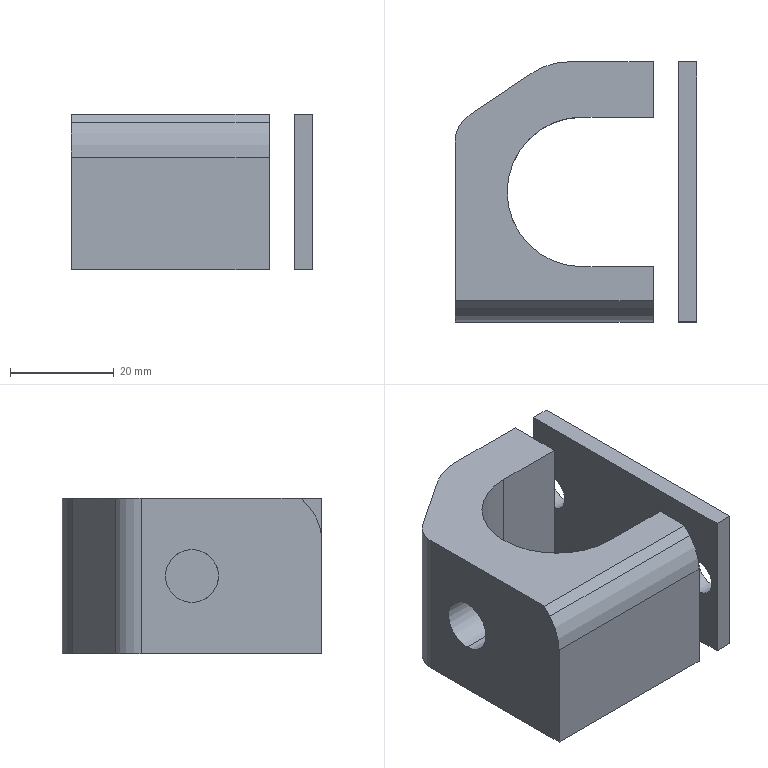Part | STEP file | SOPORTE BALANCIN | 2 solids | 36 faces | box 46.5 x 50 x 30 mm | volume 35322 mm3 | plane 17 | cylinder 15 | cone 4 | commonest cylinder face diameters 5 x4 7 x4 10.2 x2 28.8 x2 12 x1 20 x1
STEP:
#1=CARTESIAN_POINT('',(22.1,-23.5,0.));
#2=VERTEX_POINT('',#1);
#3=CARTESIAN_POINT('',(22.1,-16.5,0.));
#4=VERTEX_POINT('',#3);
#5=CARTESIAN_POINT('',(22.1,-20.,0.));
#6=DIRECTION('',(1.,0.,0.));
#7=DIRECTION('',(0.,1.,0.));
#8=AXIS2_PLACEMENT_3D('',#5,#6,#7);
#9=CIRCLE('',#8,3.5);
#10=EDGE_CURVE('',#2,#4,#9,.T.);
#11=ORIENTED_EDGE('',*,*,#10,.T.);
#12=CARTESIAN_POINT('',(18.6,-16.5,0.));
#13=VERTEX_POINT('',#12);
#14=CARTESIAN_POINT('',(22.1,-16.5,0.));
#15=DIRECTION('',(-1.,0.,0.));
#16=VECTOR('',#15,1000.);
#17=LINE('',#14,#16);
#18=EDGE_CURVE('',#4,#13,#17,.T.);
#19=ORIENTED_EDGE('',*,*,#18,.T.);
#20=CARTESIAN_POINT('',(18.6,-23.5,0.));
#21=VERTEX_POINT('',#20);
#22=CARTESIAN_POINT('',(18.6,-20.,0.));
#23=DIRECTION('',(1.,0.,0.));
#24=DIRECTION('',(0.,1.,0.));
#25=AXIS2_PLACEMENT_3D('',#22,#23,#24);
#26=CIRCLE('',#25,3.5);
#27=EDGE_CURVE('',#21,#13,#26,.T.);
#28=ORIENTED_EDGE('',*,*,#27,.F.);
#29=CARTESIAN_POINT('',(22.1,-23.5,0.));
#30=DIRECTION('',(-1.,0.,0.));
#31=VECTOR('',#30,1000.);
#32=LINE('',#29,#31);
#33=EDGE_CURVE('',#2,#21,#32,.T.);
#34=ORIENTED_EDGE('',*,*,#33,.F.);
#35=EDGE_LOOP('',(#11,#19,#28,#34));
#36=FACE_OUTER_BOUND('',#35,.T.);
#37=CARTESIAN_POINT('',(22.1,-20.,0.));
#38=DIRECTION('',(-1.,0.,0.));
#39=DIRECTION('',(0.,-1.,0.));
#40=AXIS2_PLACEMENT_3D('',#37,#38,#39);
#41=CYLINDRICAL_SURFACE('',#40,3.5);
#42=ADVANCED_FACE('',(#36),#41,.F.);
#43=CARTESIAN_POINT('',(22.1,16.5,0.));
#44=VERTEX_POINT('',#43);
#45=CARTESIAN_POINT('',(22.1,23.5,0.));
#46=VERTEX_POINT('',#45);
#47=CARTESIAN_POINT('',(22.1,20.,0.));
#48=DIRECTION('',(1.,0.,0.));
#49=DIRECTION('',(0.,1.,0.));
#50=AXIS2_PLACEMENT_3D('',#47,#48,#49);
#51=CIRCLE('',#50,3.5);
#52=EDGE_CURVE('',#44,#46,#51,.T.);
#53=ORIENTED_EDGE('',*,*,#52,.T.);
#54=CARTESIAN_POINT('',(18.6,23.5,0.));
#55=VERTEX_POINT('',#54);
#56=CARTESIAN_POINT('',(22.1,23.5,0.));
#57=DIRECTION('',(-1.,0.,0.));
#58=VECTOR('',#57,1000.);
#59=LINE('',#56,#58);
#60=EDGE_CURVE('',#46,#55,#59,.T.);
#61=ORIENTED_EDGE('',*,*,#60,.T.);
#62=CARTESIAN_POINT('',(18.6,16.5,0.));
#63=VERTEX_POINT('',#62);
#64=CARTESIAN_POINT('',(18.6,20.,0.));
#65=DIRECTION('',(1.,0.,0.));
#66=DIRECTION('',(0.,1.,0.));
#67=AXIS2_PLACEMENT_3D('',#64,#65,#66);
#68=CIRCLE('',#67,3.5);
#69=EDGE_CURVE('',#63,#55,#68,.T.);
#70=ORIENTED_EDGE('',*,*,#69,.F.);
#71=CARTESIAN_POINT('',(22.1,16.5,0.));
#72=DIRECTION('',(-1.,0.,0.));
#73=VECTOR('',#72,1000.);
#74=LINE('',#71,#73);
#75=EDGE_CURVE('',#44,#63,#74,.T.);
#76=ORIENTED_EDGE('',*,*,#75,.F.);
#77=EDGE_LOOP('',(#53,#61,#70,#76));
#78=FACE_OUTER_BOUND('',#77,.T.);
#79=CARTESIAN_POINT('',(22.1,20.,0.));
#80=DIRECTION('',(-1.,0.,0.));
#81=DIRECTION('',(0.,-1.,0.));
#82=AXIS2_PLACEMENT_3D('',#79,#80,#81);
#83=CYLINDRICAL_SURFACE('',#82,3.5);
#84=ADVANCED_FACE('',(#78),#83,.F.);
#85=CARTESIAN_POINT('',(22.1,-25.,-15.));
#86=VERTEX_POINT('',#85);
#87=CARTESIAN_POINT('',(22.1,25.,-15.));
#88=VERTEX_POINT('',#87);
#89=CARTESIAN_POINT('',(22.1,-25.,-15.));
#90=DIRECTION('',(0.,1.,0.));
#91=VECTOR('',#90,1000.);
#92=LINE('',#89,#91);
#93=EDGE_CURVE('',#86,#88,#92,.T.);
#94=ORIENTED_EDGE('',*,*,#93,.T.);
#95=CARTESIAN_POINT('',(22.1,25.,15.));
#96=VERTEX_POINT('',#95);
#97=CARTESIAN_POINT('',(22.1,25.,15.));
#98=DIRECTION('',(0.,0.,1.));
#99=VECTOR('',#98,1000.);
#100=LINE('',#97,#99);
#101=EDGE_CURVE('',#88,#96,#100,.T.);
#102=ORIENTED_EDGE('',*,*,#101,.T.);
#103=CARTESIAN_POINT('',(22.1,-25.,15.));
#104=VERTEX_POINT('',#103);
#105=CARTESIAN_POINT('',(22.1,-25.,15.));
#106=DIRECTION('',(0.,-1.,0.));
#107=VECTOR('',#106,1000.);
#108=LINE('',#105,#107);
#109=EDGE_CURVE('',#96,#104,#108,.T.);
#110=ORIENTED_EDGE('',*,*,#109,.T.);
#111=CARTESIAN_POINT('',(22.1,-25.,15.));
#112=DIRECTION('',(0.,0.,-1.));
#113=VECTOR('',#112,1000.);
#114=LINE('',#111,#113);
#115=EDGE_CURVE('',#104,#86,#114,.T.);
#116=ORIENTED_EDGE('',*,*,#115,.T.);
#117=EDGE_LOOP('',(#94,#102,#110,#116));
#118=FACE_OUTER_BOUND('',#117,.T.);
#119=ORIENTED_EDGE('',*,*,#52,.F.);
#120=CARTESIAN_POINT('',(22.1,20.,0.));
#121=DIRECTION('',(1.,0.,0.));
#122=DIRECTION('',(0.,1.,0.));
#123=AXIS2_PLACEMENT_3D('',#120,#121,#122);
#124=CIRCLE('',#123,3.5);
#125=EDGE_CURVE('',#46,#44,#124,.T.);
#126=ORIENTED_EDGE('',*,*,#125,.F.);
#127=EDGE_LOOP('',(#119,#126));
#128=FACE_BOUND('',#127,.T.);
#129=ORIENTED_EDGE('',*,*,#10,.F.);
#130=CARTESIAN_POINT('',(22.1,-20.,0.));
#131=DIRECTION('',(1.,0.,0.));
#132=DIRECTION('',(0.,1.,0.));
#133=AXIS2_PLACEMENT_3D('',#130,#131,#132);
#134=CIRCLE('',#133,3.5);
#135=EDGE_CURVE('',#4,#2,#134,.T.);
#136=ORIENTED_EDGE('',*,*,#135,.F.);
#137=EDGE_LOOP('',(#129,#136));
#138=FACE_BOUND('',#137,.T.);
#139=CARTESIAN_POINT('',(22.1,0.,0.));
#140=DIRECTION('',(-1.,0.,0.));
#141=DIRECTION('',(0.,-1.,0.));
#142=AXIS2_PLACEMENT_3D('',#139,#140,#141);
#143=PLANE('',#142);
#144=ADVANCED_FACE('',(#118,#128,#138),#143,.F.);
#145=ORIENTED_EDGE('',*,*,#69,.T.);
#146=CARTESIAN_POINT('',(18.6,20.,0.));
#147=DIRECTION('',(1.,0.,0.));
#148=DIRECTION('',(0.,1.,0.));
#149=AXIS2_PLACEMENT_3D('',#146,#147,#148);
#150=CIRCLE('',#149,3.5);
#151=EDGE_CURVE('',#55,#63,#150,.T.);
#152=ORIENTED_EDGE('',*,*,#151,.T.);
#153=EDGE_LOOP('',(#145,#152));
#154=FACE_BOUND('',#153,.T.);
#155=CARTESIAN_POINT('',(18.6,-25.,-15.));
#156=VERTEX_POINT('',#155);
#157=CARTESIAN_POINT('',(18.6,25.,-15.));
#158=VERTEX_POINT('',#157);
#159=CARTESIAN_POINT('',(18.6,-25.,-15.));
#160=DIRECTION('',(0.,1.,0.));
#161=VECTOR('',#160,1000.);
#162=LINE('',#159,#161);
#163=EDGE_CURVE('',#156,#158,#162,.T.);
#164=ORIENTED_EDGE('',*,*,#163,.F.);
#165=CARTESIAN_POINT('',(18.6,-25.,15.));
#166=VERTEX_POINT('',#165);
#167=CARTESIAN_POINT('',(18.6,-25.,15.));
#168=DIRECTION('',(0.,0.,-1.));
#169=VECTOR('',#168,1000.);
#170=LINE('',#167,#169);
#171=EDGE_CURVE('',#166,#156,#170,.T.);
#172=ORIENTED_EDGE('',*,*,#171,.F.);
#173=CARTESIAN_POINT('',(18.6,25.,15.));
#174=VERTEX_POINT('',#173);
#175=CARTESIAN_POINT('',(18.6,-25.,15.));
#176=DIRECTION('',(0.,-1.,0.));
#177=VECTOR('',#176,1000.);
#178=LINE('',#175,#177);
#179=EDGE_CURVE('',#174,#166,#178,.T.);
#180=ORIENTED_EDGE('',*,*,#179,.F.);
#181=CARTESIAN_POINT('',(18.6,25.,15.));
#182=DIRECTION('',(0.,0.,1.));
#183=VECTOR('',#182,1000.);
#184=LINE('',#181,#183);
#185=EDGE_CURVE('',#158,#174,#184,.T.);
#186=ORIENTED_EDGE('',*,*,#185,.F.);
#187=EDGE_LOOP('',(#164,#172,#180,#186));
#188=FACE_OUTER_BOUND('',#187,.T.);
#189=ORIENTED_EDGE('',*,*,#27,.T.);
#190=CARTESIAN_POINT('',(18.6,-20.,0.));
#191=DIRECTION('',(1.,0.,0.));
#192=DIRECTION('',(0.,1.,0.));
#193=AXIS2_PLACEMENT_3D('',#190,#191,#192);
#194=CIRCLE('',#193,3.5);
#195=EDGE_CURVE('',#13,#21,#194,.T.);
#196=ORIENTED_EDGE('',*,*,#195,.T.);
#197=EDGE_LOOP('',(#189,#196));
#198=FACE_BOUND('',#197,.T.);
#199=CARTESIAN_POINT('',(18.6,0.,0.));
#200=DIRECTION('',(-1.,0.,0.));
#201=DIRECTION('',(0.,-1.,0.));
#202=AXIS2_PLACEMENT_3D('',#199,#200,#201);
#203=PLANE('',#202);
#204=ADVANCED_FACE('',(#154,#188,#198),#203,.T.);
#205=ORIENTED_EDGE('',*,*,#163,.T.);
#206=CARTESIAN_POINT('',(22.1,25.,-15.));
#207=DIRECTION('',(-1.,0.,0.));
#208=VECTOR('',#207,1000.);
#209=LINE('',#206,#208);
#210=EDGE_CURVE('',#88,#158,#209,.T.);
#211=ORIENTED_EDGE('',*,*,#210,.F.);
#212=ORIENTED_EDGE('',*,*,#93,.F.);
#213=CARTESIAN_POINT('',(22.1,-25.,-15.));
#214=DIRECTION('',(-1.,0.,0.));
#215=VECTOR('',#214,1000.);
#216=LINE('',#213,#215);
#217=EDGE_CURVE('',#86,#156,#216,.T.);
#218=ORIENTED_EDGE('',*,*,#217,.T.);
#219=EDGE_LOOP('',(#205,#211,#212,#218));
#220=FACE_OUTER_BOUND('',#219,.T.);
#221=CARTESIAN_POINT('',(22.1,-25.,-15.));
#222=DIRECTION('',(0.,0.,1.));
#223=DIRECTION('',(1.,0.,0.));
#224=AXIS2_PLACEMENT_3D('',#221,#222,#223);
#225=PLANE('',#224);
#226=ADVANCED_FACE('',(#220),#225,.F.);
#227=ORIENTED_EDGE('',*,*,#185,.T.);
#228=CARTESIAN_POINT('',(22.1,25.,15.));
#229=DIRECTION('',(-1.,0.,0.));
#230=VECTOR('',#229,1000.);
#231=LINE('',#228,#230);
#232=EDGE_CURVE('',#96,#174,#231,.T.);
#233=ORIENTED_EDGE('',*,*,#232,.F.);
#234=ORIENTED_EDGE('',*,*,#101,.F.);
#235=ORIENTED_EDGE('',*,*,#210,.T.);
#236=EDGE_LOOP('',(#227,#233,#234,#235));
#237=FACE_OUTER_BOUND('',#236,.T.);
#238=CARTESIAN_POINT('',(22.1,25.,15.));
#239=DIRECTION('',(0.,-1.,0.));
#240=DIRECTION('',(1.,0.,0.));
#241=AXIS2_PLACEMENT_3D('',#238,#239,#240);
#242=PLANE('',#241);
#243=ADVANCED_FACE('',(#237),#242,.F.);
#244=ORIENTED_EDGE('',*,*,#179,.T.);
#245=CARTESIAN_POINT('',(22.1,-25.,15.));
#246=DIRECTION('',(-1.,0.,0.));
#247=VECTOR('',#246,1000.);
#248=LINE('',#245,#247);
#249=EDGE_CURVE('',#104,#166,#248,.T.);
#250=ORIENTED_EDGE('',*,*,#249,.F.);
#251=ORIENTED_EDGE('',*,*,#109,.F.);
#252=ORIENTED_EDGE('',*,*,#232,.T.);
#253=EDGE_LOOP('',(#244,#250,#251,#252));
#254=FACE_OUTER_BOUND('',#253,.T.);
#255=CARTESIAN_POINT('',(22.1,-25.,15.));
#256=DIRECTION('',(0.,0.,-1.));
#257=DIRECTION('',(-1.,0.,0.));
#258=AXIS2_PLACEMENT_3D('',#255,#256,#257);
#259=PLANE('',#258);
#260=ADVANCED_FACE('',(#254),#259,.F.);
#261=ORIENTED_EDGE('',*,*,#171,.T.);
#262=ORIENTED_EDGE('',*,*,#217,.F.);
#263=ORIENTED_EDGE('',*,*,#115,.F.);
#264=ORIENTED_EDGE('',*,*,#249,.T.);
#265=EDGE_LOOP('',(#261,#262,#263,#264));
#266=FACE_OUTER_BOUND('',#265,.T.);
#267=CARTESIAN_POINT('',(22.1,-25.,15.));
#268=DIRECTION('',(0.,1.,0.));
#269=DIRECTION('',(-1.,0.,0.));
#270=AXIS2_PLACEMENT_3D('',#267,#268,#269);
#271=PLANE('',#270);
#272=ADVANCED_FACE('',(#266),#271,.F.);
#273=ORIENTED_EDGE('',*,*,#60,.F.);
#274=ORIENTED_EDGE('',*,*,#125,.T.);
#275=ORIENTED_EDGE('',*,*,#75,.T.);
#276=ORIENTED_EDGE('',*,*,#151,.F.);
#277=EDGE_LOOP('',(#273,#274,#275,#276));
#278=FACE_OUTER_BOUND('',#277,.T.);
#279=CARTESIAN_POINT('',(22.1,20.,0.));
#280=DIRECTION('',(-1.,0.,0.));
#281=DIRECTION('',(0.,-1.,0.));
#282=AXIS2_PLACEMENT_3D('',#279,#280,#281);
#283=CYLINDRICAL_SURFACE('',#282,3.5);
#284=ADVANCED_FACE('',(#278),#283,.F.);
#285=ORIENTED_EDGE('',*,*,#18,.F.);
#286=ORIENTED_EDGE('',*,*,#135,.T.);
#287=ORIENTED_EDGE('',*,*,#33,.T.);
#288=ORIENTED_EDGE('',*,*,#195,.F.);
#289=EDGE_LOOP('',(#285,#286,#287,#288));
#290=FACE_OUTER_BOUND('',#289,.T.);
#291=CARTESIAN_POINT('',(22.1,-20.,0.));
#292=DIRECTION('',(-1.,0.,0.));
#293=DIRECTION('',(0.,-1.,0.));
#294=AXIS2_PLACEMENT_3D('',#291,#292,#293);
#295=CYLINDRICAL_SURFACE('',#294,3.5);
#296=ADVANCED_FACE('',(#290),#295,.F.);
#297=CLOSED_SHELL('',(#42,#84,#144,#204,#226,#243,#260,#272,#284,#296));
#298=MANIFOLD_SOLID_BREP('',#297);
#299=CARTESIAN_POINT('',(-14.4,0.,-5.1));
#300=VERTEX_POINT('',#299);
#301=CARTESIAN_POINT('',(-14.4,0.,5.1));
#302=VERTEX_POINT('',#301);
#303=CARTESIAN_POINT('',(-14.4,0.,-5.1));
#304=CARTESIAN_POINT('',(-14.4,-0.1674,-5.1));
#305=CARTESIAN_POINT('',(-14.397,-0.3348,-5.092));
#306=CARTESIAN_POINT('',(-14.385,-0.6696,-5.059));
#307=CARTESIAN_POINT('',(-14.377,-0.838,-5.034));
#308=CARTESIAN_POINT('',(-14.342,-1.334,-4.934));
#309=CARTESIAN_POINT('',(-14.308,-1.653,-4.836));
#310=CARTESIAN_POINT('',(-14.224,-2.269,-4.58));
#311=CARTESIAN_POINT('',(-14.172,-2.567,-4.419));
#312=CARTESIAN_POINT('',(-14.061,-3.117,-4.05));
#313=CARTESIAN_POINT('',(-14.002,-3.372,-3.84));
#314=CARTESIAN_POINT('',(-13.88,-3.843,-3.369));
#315=CARTESIAN_POINT('',(-13.819,-4.054,-3.112));
#316=CARTESIAN_POINT('',(-13.734,-4.329,-2.701));
#317=CARTESIAN_POINT('',(-13.707,-4.415,-2.559));
#318=CARTESIAN_POINT('',(-13.655,-4.572,-2.266));
#319=CARTESIAN_POINT('',(-13.631,-4.645,-2.113));
#320=CARTESIAN_POINT('',(-13.564,-4.838,-1.649));
#321=CARTESIAN_POINT('',(-13.528,-4.935,-1.331));
#322=CARTESIAN_POINT('',(-13.48,-5.066,-0.6757));
#323=CARTESIAN_POINT('',(-13.467,-5.1,-0.3347));
#324=CARTESIAN_POINT('',(-13.467,-5.1,0.3374));
#325=CARTESIAN_POINT('',(-13.479,-5.067,0.6706));
#326=CARTESIAN_POINT('',(-13.516,-4.968,1.166));
#327=CARTESIAN_POINT('',(-13.531,-4.926,1.331));
#328=CARTESIAN_POINT('',(-13.567,-4.828,1.651));
#329=CARTESIAN_POINT('',(-13.587,-4.772,1.808));
#330=CARTESIAN_POINT('',(-13.653,-4.58,2.269));
#331=CARTESIAN_POINT('',(-13.706,-4.421,2.565));
#332=CARTESIAN_POINT('',(-13.82,-4.05,3.118));
#333=CARTESIAN_POINT('',(-13.881,-3.84,3.373));
#334=CARTESIAN_POINT('',(-14.002,-3.372,3.84));
#335=CARTESIAN_POINT('',(-14.062,-3.112,4.054));
#336=CARTESIAN_POINT('',(-14.173,-2.562,4.422));
#337=CARTESIAN_POINT('',(-14.223,-2.27,4.579));
#338=CARTESIAN_POINT('',(-14.287,-1.807,4.772));
#339=CARTESIAN_POINT('',(-14.306,-1.647,4.83));
#340=CARTESIAN_POINT('',(-14.34,-1.326,4.927));
#341=CARTESIAN_POINT('',(-14.354,-1.164,4.968));
#342=CARTESIAN_POINT('',(-14.388,-0.6735,5.066));
#343=CARTESIAN_POINT('',(-14.4,-0.3399,5.1));
#344=CARTESIAN_POINT('',(-14.4,0.,5.1));
#345=B_SPLINE_CURVE_WITH_KNOTS('',3,(#303,#304,#305,#306,#307,#308,#309,#310,#311,#312,#313,#314,#315,#316,#317,#318,#319,#320,#321,#322,#323,#324,#325,#326,#327,#328,#329,#330,#331,#332,#333,#334,#335,#336,#337,#338,#339,#340,#341,#342,#343,#344),.UNSPECIFIED.,.F.,.F.,(4,2,2,2,2,2,2,2,2,2,2,2,2,2,2,2,2,2,2,2,4),(0.01608,0.01658,0.01708,0.01809,0.01909,0.02009,0.0211,0.0216,0.0221,0.02311,0.02411,0.02512,0.02562,0.02612,0.02713,0.02813,0.02914,0.03014,0.03064,0.03114,0.03215),.UNSPECIFIED.);
#346=EDGE_CURVE('',#300,#302,#345,.T.);
#347=ORIENTED_EDGE('',*,*,#346,.F.);
#348=CARTESIAN_POINT('',(-24.4,0.,-5.1));
#349=VERTEX_POINT('',#348);
#350=CARTESIAN_POINT('',(-24.4,0.,-5.1));
#351=DIRECTION('',(-1.,0.,0.));
#352=VECTOR('',#351,1000.);
#353=LINE('',#350,#352);
#354=EDGE_CURVE('',#300,#349,#353,.T.);
#355=ORIENTED_EDGE('',*,*,#354,.T.);
#356=CARTESIAN_POINT('',(-24.4,0.,5.1));
#357=VERTEX_POINT('',#356);
#358=CARTESIAN_POINT('',(-24.4,0.,0.));
#359=DIRECTION('',(-1.,0.,0.));
#360=DIRECTION('',(0.,0.,1.));
#361=AXIS2_PLACEMENT_3D('',#358,#359,#360);
#362=CIRCLE('',#361,5.1);
#363=EDGE_CURVE('',#349,#357,#362,.T.);
#364=ORIENTED_EDGE('',*,*,#363,.T.);
#365=CARTESIAN_POINT('',(-24.4,0.,5.1));
#366=DIRECTION('',(-1.,0.,0.));
#367=VECTOR('',#366,1000.);
#368=LINE('',#365,#367);
#369=EDGE_CURVE('',#302,#357,#368,.T.);
#370=ORIENTED_EDGE('',*,*,#369,.F.);
#371=EDGE_LOOP('',(#347,#355,#364,#370));
#372=FACE_OUTER_BOUND('',#371,.T.);
#373=CARTESIAN_POINT('',(-24.4,0.,0.));
#374=DIRECTION('',(-1.,0.,0.));
#375=DIRECTION('',(0.,0.,1.));
#376=AXIS2_PLACEMENT_3D('',#373,#374,#375);
#377=CYLINDRICAL_SURFACE('',#376,5.1);
#378=ADVANCED_FACE('',(#372),#377,.F.);
#379=CARTESIAN_POINT('',(-1.898,20.,2.5));
#380=VERTEX_POINT('',#379);
#381=CARTESIAN_POINT('',(-1.898,20.,-2.5));
#382=VERTEX_POINT('',#381);
#383=CARTESIAN_POINT('',(-1.898,20.,0.));
#384=DIRECTION('',(1.,0.,0.));
#385=DIRECTION('',(0.,0.,-1.));
#386=AXIS2_PLACEMENT_3D('',#383,#384,#385);
#387=CIRCLE('',#386,2.5);
#388=EDGE_CURVE('',#380,#382,#387,.T.);
#389=ORIENTED_EDGE('',*,*,#388,.F.);
#390=CARTESIAN_POINT('',(13.7,20.,2.5));
#391=VERTEX_POINT('',#390);
#392=CARTESIAN_POINT('',(13.6,20.,2.5));
#393=DIRECTION('',(1.,0.,0.));
#394=VECTOR('',#393,1000.);
#395=LINE('',#392,#394);
#396=EDGE_CURVE('',#380,#391,#395,.T.);
#397=ORIENTED_EDGE('',*,*,#396,.T.);
#398=CARTESIAN_POINT('',(13.7,20.,-2.5));
#399=VERTEX_POINT('',#398);
#400=CARTESIAN_POINT('',(13.7,20.,0.));
#401=DIRECTION('',(1.,0.,0.));
#402=DIRECTION('',(0.,-1.,0.));
#403=AXIS2_PLACEMENT_3D('',#400,#401,#402);
#404=CIRCLE('',#403,2.5);
#405=EDGE_CURVE('',#391,#399,#404,.T.);
#406=ORIENTED_EDGE('',*,*,#405,.T.);
#407=CARTESIAN_POINT('',(13.6,20.,-2.5));
#408=DIRECTION('',(1.,0.,0.));
#409=VECTOR('',#408,1000.);
#410=LINE('',#407,#409);
#411=EDGE_CURVE('',#382,#399,#410,.T.);
#412=ORIENTED_EDGE('',*,*,#411,.F.);
#413=EDGE_LOOP('',(#389,#397,#406,#412));
#414=FACE_OUTER_BOUND('',#413,.T.);
#415=CARTESIAN_POINT('',(13.6,20.,0.));
#416=DIRECTION('',(1.,0.,0.));
#417=DIRECTION('',(0.,0.,-1.));
#418=AXIS2_PLACEMENT_3D('',#415,#416,#417);
#419=CYLINDRICAL_SURFACE('',#418,2.5);
#420=ADVANCED_FACE('',(#414),#419,.F.);
#421=CARTESIAN_POINT('',(-3.4,20.,0.));
#422=VERTEX_POINT('',#421);
#423=CARTESIAN_POINT('',(-1.898,20.,-2.5));
#424=DIRECTION('',(0.515,0.,-0.8572));
#425=VECTOR('',#424,1000.);
#426=LINE('',#423,#425);
#427=EDGE_CURVE('',#422,#382,#426,.T.);
#428=ORIENTED_EDGE('',*,*,#427,.F.);
#429=CARTESIAN_POINT('',(-1.898,20.,2.5));
#430=DIRECTION('',(0.515,0.,0.8572));
#431=VECTOR('',#430,1000.);
#432=LINE('',#429,#431);
#433=EDGE_CURVE('',#422,#380,#432,.T.);
#434=ORIENTED_EDGE('',*,*,#433,.T.);
#435=ORIENTED_EDGE('',*,*,#388,.T.);
#436=EDGE_LOOP('',(#428,#434,#435));
#437=FACE_OUTER_BOUND('',#436,.T.);
#438=CARTESIAN_POINT('',(-1.898,20.,0.));
#439=DIRECTION('',(1.,0.,0.));
#440=DIRECTION('',(0.,0.,-1.));
#441=AXIS2_PLACEMENT_3D('',#438,#439,#440);
#442=CONICAL_SURFACE('',#441,2.5,1.03);
#443=ADVANCED_FACE('',(#437),#442,.F.);
#444=CARTESIAN_POINT('',(-1.898,-20.,2.5));
#445=VERTEX_POINT('',#444);
#446=CARTESIAN_POINT('',(-1.898,-20.,-2.5));
#447=VERTEX_POINT('',#446);
#448=CARTESIAN_POINT('',(-1.898,-20.,0.));
#449=DIRECTION('',(1.,0.,0.));
#450=DIRECTION('',(0.,0.,-1.));
#451=AXIS2_PLACEMENT_3D('',#448,#449,#450);
#452=CIRCLE('',#451,2.5);
#453=EDGE_CURVE('',#445,#447,#452,.T.);
#454=ORIENTED_EDGE('',*,*,#453,.F.);
#455=CARTESIAN_POINT('',(13.7,-20.,2.5));
#456=VERTEX_POINT('',#455);
#457=CARTESIAN_POINT('',(13.6,-20.,2.5));
#458=DIRECTION('',(1.,0.,0.));
#459=VECTOR('',#458,1000.);
#460=LINE('',#457,#459);
#461=EDGE_CURVE('',#445,#456,#460,.T.);
#462=ORIENTED_EDGE('',*,*,#461,.T.);
#463=CARTESIAN_POINT('',(13.7,-20.,-2.5));
#464=VERTEX_POINT('',#463);
#465=CARTESIAN_POINT('',(13.7,-20.,0.));
#466=DIRECTION('',(1.,0.,0.));
#467=DIRECTION('',(0.,-1.,0.));
#468=AXIS2_PLACEMENT_3D('',#465,#466,#467);
#469=CIRCLE('',#468,2.5);
#470=EDGE_CURVE('',#456,#464,#469,.T.);
#471=ORIENTED_EDGE('',*,*,#470,.T.);
#472=CARTESIAN_POINT('',(13.6,-20.,-2.5));
#473=DIRECTION('',(1.,0.,0.));
#474=VECTOR('',#473,1000.);
#475=LINE('',#472,#474);
#476=EDGE_CURVE('',#447,#464,#475,.T.);
#477=ORIENTED_EDGE('',*,*,#476,.F.);
#478=EDGE_LOOP('',(#454,#462,#471,#477));
#479=FACE_OUTER_BOUND('',#478,.T.);
#480=CARTESIAN_POINT('',(13.6,-20.,0.));
#481=DIRECTION('',(1.,0.,0.));
#482=DIRECTION('',(0.,0.,-1.));
#483=AXIS2_PLACEMENT_3D('',#480,#481,#482);
#484=CYLINDRICAL_SURFACE('',#483,2.5);
#485=ADVANCED_FACE('',(#479),#484,.F.);
#486=CARTESIAN_POINT('',(-3.4,-20.,0.));
#487=VERTEX_POINT('',#486);
#488=CARTESIAN_POINT('',(-1.898,-20.,-2.5));
#489=DIRECTION('',(0.515,0.,-0.8572));
#490=VECTOR('',#489,1000.);
#491=LINE('',#488,#490);
#492=EDGE_CURVE('',#487,#447,#491,.T.);
#493=ORIENTED_EDGE('',*,*,#492,.F.);
#494=CARTESIAN_POINT('',(-1.898,-20.,2.5));
#495=DIRECTION('',(0.515,0.,0.8572));
#496=VECTOR('',#495,1000.);
#497=LINE('',#494,#496);
#498=EDGE_CURVE('',#487,#445,#497,.T.);
#499=ORIENTED_EDGE('',*,*,#498,.T.);
#500=ORIENTED_EDGE('',*,*,#453,.T.);
#501=EDGE_LOOP('',(#493,#499,#500));
#502=FACE_OUTER_BOUND('',#501,.T.);
#503=CARTESIAN_POINT('',(-1.898,-20.,0.));
#504=DIRECTION('',(1.,0.,0.));
#505=DIRECTION('',(0.,0.,-1.));
#506=AXIS2_PLACEMENT_3D('',#503,#504,#505);
#507=CONICAL_SURFACE('',#506,2.5,1.03);
#508=ADVANCED_FACE('',(#502),#507,.F.);
#509=CARTESIAN_POINT('',(-14.4,0.,15.));
#510=VERTEX_POINT('',#509);
#511=CARTESIAN_POINT('',(0.,14.4,15.));
#512=VERTEX_POINT('',#511);
#513=CARTESIAN_POINT('',(0.,0.,15.));
#514=DIRECTION('',(0.,0.,-1.));
#515=DIRECTION('',(1.,0.,0.));
#516=AXIS2_PLACEMENT_3D('',#513,#514,#515);
#517=CIRCLE('',#516,14.4);
#518=EDGE_CURVE('',#510,#512,#517,.T.);
#519=ORIENTED_EDGE('',*,*,#518,.F.);
#520=CARTESIAN_POINT('',(-14.4,0.,15.));
#521=DIRECTION('',(0.,0.,-1.));
#522=VECTOR('',#521,1000.);
#523=LINE('',#520,#522);
#524=EDGE_CURVE('',#510,#302,#523,.T.);
#525=ORIENTED_EDGE('',*,*,#524,.T.);
#526=CARTESIAN_POINT('',(-14.4,0.,5.1));
#527=CARTESIAN_POINT('',(-14.4,0.3399,5.1));
#528=CARTESIAN_POINT('',(-14.388,0.6737,5.066));
#529=CARTESIAN_POINT('',(-14.342,1.329,4.935));
#530=CARTESIAN_POINT('',(-14.308,1.655,4.836));
#531=CARTESIAN_POINT('',(-14.223,2.271,4.578));
#532=CARTESIAN_POINT('',(-14.173,2.563,4.421));
#533=CARTESIAN_POINT('',(-14.062,3.116,4.051));
#534=CARTESIAN_POINT('',(-14.001,3.375,3.838));
#535=CARTESIAN_POINT('',(-13.88,3.841,3.371));
#536=CARTESIAN_POINT('',(-13.82,4.051,3.116));
#537=CARTESIAN_POINT('',(-13.705,4.424,2.56));
#538=CARTESIAN_POINT('',(-13.653,4.58,2.268));
#539=CARTESIAN_POINT('',(-13.587,4.772,1.808));
#540=CARTESIAN_POINT('',(-13.567,4.828,1.652));
#541=CARTESIAN_POINT('',(-13.531,4.926,1.331));
#542=CARTESIAN_POINT('',(-13.516,4.968,1.166));
#543=CARTESIAN_POINT('',(-13.479,5.067,0.6712));
#544=CARTESIAN_POINT('',(-13.467,5.1,0.3384));
#545=CARTESIAN_POINT('',(-13.467,5.1,-0.3331));
#546=CARTESIAN_POINT('',(-13.48,5.066,-0.6741));
#547=CARTESIAN_POINT('',(-13.528,4.935,-1.331));
#548=CARTESIAN_POINT('',(-13.564,4.837,-1.65));
#549=CARTESIAN_POINT('',(-13.653,4.579,-2.271));
#550=CARTESIAN_POINT('',(-13.706,4.421,-2.564));
#551=CARTESIAN_POINT('',(-13.819,4.053,-3.114));
#552=CARTESIAN_POINT('',(-13.881,3.839,-3.373));
#553=CARTESIAN_POINT('',(-14.002,3.37,-3.842));
#554=CARTESIAN_POINT('',(-14.062,3.116,-4.051));
#555=CARTESIAN_POINT('',(-14.173,2.565,-4.421));
#556=CARTESIAN_POINT('',(-14.224,2.266,-4.581));
#557=CARTESIAN_POINT('',(-14.308,1.653,-4.836));
#558=CARTESIAN_POINT('',(-14.342,1.334,-4.934));
#559=CARTESIAN_POINT('',(-14.377,0.838,-5.034));
#560=CARTESIAN_POINT('',(-14.385,0.6696,-5.059));
#561=CARTESIAN_POINT('',(-14.397,0.3348,-5.092));
#562=CARTESIAN_POINT('',(-14.4,0.1674,-5.1));
#563=CARTESIAN_POINT('',(-14.4,0.,-5.1));
#564=B_SPLINE_CURVE_WITH_KNOTS('',3,(#526,#527,#528,#529,#530,#531,#532,#533,#534,#535,#536,#537,#538,#539,#540,#541,#542,#543,#544,#545,#546,#547,#548,#549,#550,#551,#552,#553,#554,#555,#556,#557,#558,#559,#560,#561,#562,#563),.UNSPECIFIED.,.F.,.F.,(4,2,2,2,2,2,2,2,2,2,2,2,2,2,2,2,2,2,4),(0.,0.001005,0.00201,0.003014,0.004019,0.005024,0.006029,0.006531,0.007033,0.008038,0.009043,0.01005,0.01105,0.01206,0.01306,0.01407,0.01507,0.01557,0.01608),.UNSPECIFIED.);
#565=EDGE_CURVE('',#302,#300,#564,.T.);
#566=ORIENTED_EDGE('',*,*,#565,.T.);
#567=CARTESIAN_POINT('',(-14.4,0.,-15.));
#568=VERTEX_POINT('',#567);
#569=CARTESIAN_POINT('',(-14.4,0.,15.));
#570=DIRECTION('',(0.,0.,-1.));
#571=VECTOR('',#570,1000.);
#572=LINE('',#569,#571);
#573=EDGE_CURVE('',#300,#568,#572,.T.);
#574=ORIENTED_EDGE('',*,*,#573,.T.);
#575=CARTESIAN_POINT('',(0.,14.4,-15.));
#576=VERTEX_POINT('',#575);
#577=CARTESIAN_POINT('',(0.,0.,-15.));
#578=DIRECTION('',(0.,0.,-1.));
#579=DIRECTION('',(1.,0.,0.));
#580=AXIS2_PLACEMENT_3D('',#577,#578,#579);
#581=CIRCLE('',#580,14.4);
#582=EDGE_CURVE('',#568,#576,#581,.T.);
#583=ORIENTED_EDGE('',*,*,#582,.T.);
#584=CARTESIAN_POINT('',(0.,14.4,15.));
#585=DIRECTION('',(0.,0.,-1.));
#586=VECTOR('',#585,1000.);
#587=LINE('',#584,#586);
#588=EDGE_CURVE('',#512,#576,#587,.T.);
#589=ORIENTED_EDGE('',*,*,#588,.F.);
#590=EDGE_LOOP('',(#519,#525,#566,#574,#583,#589));
#591=FACE_OUTER_BOUND('',#590,.T.);
#592=CARTESIAN_POINT('',(0.,0.,15.));
#593=DIRECTION('',(0.,0.,-1.));
#594=DIRECTION('',(-1.,0.,0.));
#595=AXIS2_PLACEMENT_3D('',#592,#593,#594);
#596=CYLINDRICAL_SURFACE('',#595,14.4);
#597=ADVANCED_FACE('',(#591),#596,.F.);
#598=CARTESIAN_POINT('',(13.7,-14.4,-15.));
#599=VERTEX_POINT('',#598);
#600=CARTESIAN_POINT('',(0.,-14.4,-15.));
#601=VERTEX_POINT('',#600);
#602=CARTESIAN_POINT('',(13.6,-14.4,-15.));
#603=DIRECTION('',(-1.,0.,0.));
#604=VECTOR('',#603,1000.);
#605=LINE('',#602,#604);
#606=EDGE_CURVE('',#599,#601,#605,.T.);
#607=ORIENTED_EDGE('',*,*,#606,.T.);
#608=CARTESIAN_POINT('',(0.,-14.4,15.));
#609=VERTEX_POINT('',#608);
#610=CARTESIAN_POINT('',(0.,-14.4,15.));
#611=DIRECTION('',(0.,0.,-1.));
#612=VECTOR('',#611,1000.);
#613=LINE('',#610,#612);
#614=EDGE_CURVE('',#609,#601,#613,.T.);
#615=ORIENTED_EDGE('',*,*,#614,.F.);
#616=CARTESIAN_POINT('',(13.7,-14.4,15.));
#617=VERTEX_POINT('',#616);
#618=CARTESIAN_POINT('',(13.6,-14.4,15.));
#619=DIRECTION('',(-1.,0.,0.));
#620=VECTOR('',#619,1000.);
#621=LINE('',#618,#620);
#622=EDGE_CURVE('',#617,#609,#621,.T.);
#623=ORIENTED_EDGE('',*,*,#622,.F.);
#624=CARTESIAN_POINT('',(13.7,-14.4,15.));
#625=DIRECTION('',(0.,0.,-1.));
#626=VECTOR('',#625,1000.);
#627=LINE('',#624,#626);
#628=EDGE_CURVE('',#617,#599,#627,.T.);
#629=ORIENTED_EDGE('',*,*,#628,.T.);
#630=EDGE_LOOP('',(#607,#615,#623,#629));
#631=FACE_OUTER_BOUND('',#630,.T.);
#632=CARTESIAN_POINT('',(13.6,-14.4,15.));
#633=DIRECTION('',(0.,-1.,0.));
#634=DIRECTION('',(1.,0.,0.));
#635=AXIS2_PLACEMENT_3D('',#632,#633,#634);
#636=PLANE('',#635);
#637=ADVANCED_FACE('',(#631),#636,.F.);
#638=ORIENTED_EDGE('',*,*,#524,.F.);
#639=CARTESIAN_POINT('',(0.,0.,15.));
#640=DIRECTION('',(0.,0.,-1.));
#641=DIRECTION('',(1.,0.,0.));
#642=AXIS2_PLACEMENT_3D('',#639,#640,#641);
#643=CIRCLE('',#642,14.4);
#644=EDGE_CURVE('',#609,#510,#643,.T.);
#645=ORIENTED_EDGE('',*,*,#644,.F.);
#646=ORIENTED_EDGE('',*,*,#614,.T.);
#647=CARTESIAN_POINT('',(0.,0.,-15.));
#648=DIRECTION('',(0.,0.,-1.));
#649=DIRECTION('',(1.,0.,0.));
#650=AXIS2_PLACEMENT_3D('',#647,#648,#649);
#651=CIRCLE('',#650,14.4);
#652=EDGE_CURVE('',#601,#568,#651,.T.);
#653=ORIENTED_EDGE('',*,*,#652,.T.);
#654=ORIENTED_EDGE('',*,*,#573,.F.);
#655=ORIENTED_EDGE('',*,*,#346,.T.);
#656=EDGE_LOOP('',(#638,#645,#646,#653,#654,#655));
#657=FACE_OUTER_BOUND('',#656,.T.);
#658=CARTESIAN_POINT('',(0.,0.,15.));
#659=DIRECTION('',(0.,0.,-1.));
#660=DIRECTION('',(-1.,0.,0.));
#661=AXIS2_PLACEMENT_3D('',#658,#659,#660);
#662=CYLINDRICAL_SURFACE('',#661,14.4);
#663=ADVANCED_FACE('',(#657),#662,.F.);
#664=CARTESIAN_POINT('',(13.7,14.4,-15.));
#665=VERTEX_POINT('',#664);
#666=CARTESIAN_POINT('',(13.6,14.4,-15.));
#667=DIRECTION('',(1.,0.,0.));
#668=VECTOR('',#667,1000.);
#669=LINE('',#666,#668);
#670=EDGE_CURVE('',#576,#665,#669,.T.);
#671=ORIENTED_EDGE('',*,*,#670,.T.);
#672=CARTESIAN_POINT('',(13.7,14.4,15.));
#673=VERTEX_POINT('',#672);
#674=CARTESIAN_POINT('',(13.7,14.4,15.));
#675=DIRECTION('',(0.,0.,-1.));
#676=VECTOR('',#675,1000.);
#677=LINE('',#674,#676);
#678=EDGE_CURVE('',#673,#665,#677,.T.);
#679=ORIENTED_EDGE('',*,*,#678,.F.);
#680=CARTESIAN_POINT('',(13.6,14.4,15.));
#681=DIRECTION('',(1.,0.,0.));
#682=VECTOR('',#681,1000.);
#683=LINE('',#680,#682);
#684=EDGE_CURVE('',#512,#673,#683,.T.);
#685=ORIENTED_EDGE('',*,*,#684,.F.);
#686=ORIENTED_EDGE('',*,*,#588,.T.);
#687=EDGE_LOOP('',(#671,#679,#685,#686));
#688=FACE_OUTER_BOUND('',#687,.T.);
#689=CARTESIAN_POINT('',(13.6,14.4,15.));
#690=DIRECTION('',(0.,1.,0.));
#691=DIRECTION('',(-1.,0.,0.));
#692=AXIS2_PLACEMENT_3D('',#689,#690,#691);
#693=PLANE('',#692);
#694=ADVANCED_FACE('',(#688),#693,.F.);
#695=CARTESIAN_POINT('',(13.7,20.,0.));
#696=DIRECTION('',(1.,0.,0.));
#697=DIRECTION('',(0.,-1.,0.));
#698=AXIS2_PLACEMENT_3D('',#695,#696,#697);
#699=CIRCLE('',#698,2.5);
#700=EDGE_CURVE('',#399,#391,#699,.T.);
#701=ORIENTED_EDGE('',*,*,#700,.F.);
#702=ORIENTED_EDGE('',*,*,#405,.F.);
#703=EDGE_LOOP('',(#701,#702));
#704=FACE_BOUND('',#703,.T.);
#705=CARTESIAN_POINT('',(13.7,25.,-15.));
#706=VERTEX_POINT('',#705);
#707=CARTESIAN_POINT('',(13.7,25.,-15.));
#708=DIRECTION('',(0.,1.,0.));
#709=VECTOR('',#708,1000.);
#710=LINE('',#707,#709);
#711=EDGE_CURVE('',#665,#706,#710,.T.);
#712=ORIENTED_EDGE('',*,*,#711,.T.);
#713=CARTESIAN_POINT('',(13.7,25.,15.));
#714=VERTEX_POINT('',#713);
#715=CARTESIAN_POINT('',(13.7,25.,15.));
#716=DIRECTION('',(0.,0.,-1.));
#717=VECTOR('',#716,1000.);
#718=LINE('',#715,#717);
#719=EDGE_CURVE('',#714,#706,#718,.T.);
#720=ORIENTED_EDGE('',*,*,#719,.F.);
#721=CARTESIAN_POINT('',(13.7,25.,15.));
#722=DIRECTION('',(0.,1.,0.));
#723=VECTOR('',#722,1000.);
#724=LINE('',#721,#723);
#725=EDGE_CURVE('',#673,#714,#724,.T.);
#726=ORIENTED_EDGE('',*,*,#725,.F.);
#727=ORIENTED_EDGE('',*,*,#678,.T.);
#728=EDGE_LOOP('',(#712,#720,#726,#727));
#729=FACE_OUTER_BOUND('',#728,.T.);
#730=CARTESIAN_POINT('',(13.7,25.,15.));
#731=DIRECTION('',(-1.,0.,0.));
#732=DIRECTION('',(0.,-1.,0.));
#733=AXIS2_PLACEMENT_3D('',#730,#731,#732);
#734=PLANE('',#733);
#735=ADVANCED_FACE('',(#704,#729),#734,.F.);
#736=CARTESIAN_POINT('',(-2.767,25.,-15.));
#737=VERTEX_POINT('',#736);
#738=CARTESIAN_POINT('',(13.6,25.,-15.));
#739=DIRECTION('',(-1.,0.,0.));
#740=VECTOR('',#739,1000.);
#741=LINE('',#738,#740);
#742=EDGE_CURVE('',#706,#737,#741,.T.);
#743=ORIENTED_EDGE('',*,*,#742,.T.);
#744=CARTESIAN_POINT('',(-2.767,25.,15.));
#745=VERTEX_POINT('',#744);
#746=CARTESIAN_POINT('',(-2.767,25.,15.));
#747=DIRECTION('',(0.,0.,1.));
#748=VECTOR('',#747,1000.);
#749=LINE('',#746,#748);
#750=EDGE_CURVE('',#737,#745,#749,.T.);
#751=ORIENTED_EDGE('',*,*,#750,.T.);
#752=CARTESIAN_POINT('',(13.6,25.,15.));
#753=DIRECTION('',(-1.,0.,0.));
#754=VECTOR('',#753,1000.);
#755=LINE('',#752,#754);
#756=EDGE_CURVE('',#714,#745,#755,.T.);
#757=ORIENTED_EDGE('',*,*,#756,.F.);
#758=ORIENTED_EDGE('',*,*,#719,.T.);
#759=EDGE_LOOP('',(#743,#751,#757,#758));
#760=FACE_OUTER_BOUND('',#759,.T.);
#761=CARTESIAN_POINT('',(13.6,25.,15.));
#762=DIRECTION('',(0.,-1.,0.));
#763=DIRECTION('',(0.,0.,-1.));
#764=AXIS2_PLACEMENT_3D('',#761,#762,#763);
#765=PLANE('',#764);
#766=ADVANCED_FACE('',(#760),#765,.F.);
#767=CARTESIAN_POINT('',(-24.4,0.,0.));
#768=DIRECTION('',(-1.,0.,0.));
#769=DIRECTION('',(0.,0.,1.));
#770=AXIS2_PLACEMENT_3D('',#767,#768,#769);
#771=CIRCLE('',#770,5.1);
#772=EDGE_CURVE('',#357,#349,#771,.T.);
#773=ORIENTED_EDGE('',*,*,#772,.F.);
#774=ORIENTED_EDGE('',*,*,#363,.F.);
#775=EDGE_LOOP('',(#773,#774));
#776=FACE_BOUND('',#775,.T.);
#777=CARTESIAN_POINT('',(-24.4,-25.,6.698));
#778=VERTEX_POINT('',#777);
#779=CARTESIAN_POINT('',(-24.4,-25.,-15.));
#780=VERTEX_POINT('',#779);
#781=CARTESIAN_POINT('',(-24.4,-25.,15.));
#782=DIRECTION('',(0.,0.,-1.));
#783=VECTOR('',#782,1000.);
#784=LINE('',#781,#783);
#785=EDGE_CURVE('',#778,#780,#784,.T.);
#786=ORIENTED_EDGE('',*,*,#785,.F.);
#787=CARTESIAN_POINT('',(-24.4,-22.474,13.342));
#788=VERTEX_POINT('',#787);
#789=CARTESIAN_POINT('',(-24.4,-15.,6.698));
#790=DIRECTION('',(-1.,0.,0.));
#791=DIRECTION('',(0.,1.,0.));
#792=AXIS2_PLACEMENT_3D('',#789,#790,#791);
#793=CIRCLE('',#792,10.);
#794=EDGE_CURVE('',#778,#788,#793,.T.);
#795=ORIENTED_EDGE('',*,*,#794,.T.);
#796=CARTESIAN_POINT('',(-24.4,-21.,15.));
#797=VERTEX_POINT('',#796);
#798=CARTESIAN_POINT('',(-24.4,-21.,15.));
#799=DIRECTION('',(0.,0.6644,0.7474));
#800=VECTOR('',#799,1000.);
#801=LINE('',#798,#800);
#802=EDGE_CURVE('',#788,#797,#801,.T.);
#803=ORIENTED_EDGE('',*,*,#802,.T.);
#804=CARTESIAN_POINT('',(-24.4,9.789,15.));
#805=VERTEX_POINT('',#804);
#806=CARTESIAN_POINT('',(-24.4,25.,15.));
#807=DIRECTION('',(0.,-1.,0.));
#808=VECTOR('',#807,1000.);
#809=LINE('',#806,#808);
#810=EDGE_CURVE('',#805,#797,#809,.T.);
#811=ORIENTED_EDGE('',*,*,#810,.F.);
#812=CARTESIAN_POINT('',(-24.4,9.789,-15.));
#813=VERTEX_POINT('',#812);
#814=CARTESIAN_POINT('',(-24.4,9.789,-15.));
#815=DIRECTION('',(0.,0.,-1.));
#816=VECTOR('',#815,1000.);
#817=LINE('',#814,#816);
#818=EDGE_CURVE('',#805,#813,#817,.T.);
#819=ORIENTED_EDGE('',*,*,#818,.T.);
#820=CARTESIAN_POINT('',(-24.4,25.,-15.));
#821=DIRECTION('',(0.,-1.,0.));
#822=VECTOR('',#821,1000.);
#823=LINE('',#820,#822);
#824=EDGE_CURVE('',#813,#780,#823,.T.);
#825=ORIENTED_EDGE('',*,*,#824,.T.);
#826=EDGE_LOOP('',(#786,#795,#803,#811,#819,#825));
#827=FACE_OUTER_BOUND('',#826,.T.);
#828=CARTESIAN_POINT('',(-24.4,25.,15.));
#829=DIRECTION('',(1.,0.,0.));
#830=DIRECTION('',(0.,1.,0.));
#831=AXIS2_PLACEMENT_3D('',#828,#829,#830);
#832=PLANE('',#831);
#833=ADVANCED_FACE('',(#776,#827),#832,.F.);
#834=CARTESIAN_POINT('',(13.7,-25.,6.698));
#835=VERTEX_POINT('',#834);
#836=CARTESIAN_POINT('',(13.7,-25.,-15.));
#837=VERTEX_POINT('',#836);
#838=CARTESIAN_POINT('',(13.7,-25.,15.));
#839=DIRECTION('',(0.,0.,-1.));
#840=VECTOR('',#839,1000.);
#841=LINE('',#838,#840);
#842=EDGE_CURVE('',#835,#837,#841,.T.);
#843=ORIENTED_EDGE('',*,*,#842,.F.);
#844=CARTESIAN_POINT('',(-24.4,-25.,6.698));
#845=DIRECTION('',(-1.,0.,0.));
#846=VECTOR('',#845,1000.);
#847=LINE('',#844,#846);
#848=EDGE_CURVE('',#835,#778,#847,.T.);
#849=ORIENTED_EDGE('',*,*,#848,.T.);
#850=ORIENTED_EDGE('',*,*,#785,.T.);
#851=CARTESIAN_POINT('',(-24.4,-25.,-15.));
#852=DIRECTION('',(1.,0.,0.));
#853=VECTOR('',#852,1000.);
#854=LINE('',#851,#853);
#855=EDGE_CURVE('',#780,#837,#854,.T.);
#856=ORIENTED_EDGE('',*,*,#855,.T.);
#857=EDGE_LOOP('',(#843,#849,#850,#856));
#858=FACE_OUTER_BOUND('',#857,.T.);
#859=CARTESIAN_POINT('',(-24.4,-25.,15.));
#860=DIRECTION('',(0.,1.,0.));
#861=DIRECTION('',(-1.,0.,0.));
#862=AXIS2_PLACEMENT_3D('',#859,#860,#861);
#863=PLANE('',#862);
#864=ADVANCED_FACE('',(#858),#863,.F.);
#865=CARTESIAN_POINT('',(13.7,-20.,0.));
#866=DIRECTION('',(1.,0.,0.));
#867=DIRECTION('',(0.,-1.,0.));
#868=AXIS2_PLACEMENT_3D('',#865,#866,#867);
#869=CIRCLE('',#868,2.5);
#870=EDGE_CURVE('',#464,#456,#869,.T.);
#871=ORIENTED_EDGE('',*,*,#870,.F.);
#872=ORIENTED_EDGE('',*,*,#470,.F.);
#873=EDGE_LOOP('',(#871,#872));
#874=FACE_BOUND('',#873,.T.);
#875=CARTESIAN_POINT('',(13.7,-21.,15.));
#876=VERTEX_POINT('',#875);
#877=CARTESIAN_POINT('',(13.7,-22.474,13.342));
#878=VERTEX_POINT('',#877);
#879=CARTESIAN_POINT('',(13.7,-21.,15.));
#880=DIRECTION('',(0.,-0.6644,-0.7474));
#881=VECTOR('',#880,1000.);
#882=LINE('',#879,#881);
#883=EDGE_CURVE('',#876,#878,#882,.T.);
#884=ORIENTED_EDGE('',*,*,#883,.T.);
#885=CARTESIAN_POINT('',(13.7,-15.,6.698));
#886=DIRECTION('',(1.,0.,0.));
#887=DIRECTION('',(0.,-1.,0.));
#888=AXIS2_PLACEMENT_3D('',#885,#886,#887);
#889=CIRCLE('',#888,10.);
#890=EDGE_CURVE('',#878,#835,#889,.T.);
#891=ORIENTED_EDGE('',*,*,#890,.T.);
#892=ORIENTED_EDGE('',*,*,#842,.T.);
#893=CARTESIAN_POINT('',(13.7,-25.,-15.));
#894=DIRECTION('',(0.,1.,0.));
#895=VECTOR('',#894,1000.);
#896=LINE('',#893,#895);
#897=EDGE_CURVE('',#837,#599,#896,.T.);
#898=ORIENTED_EDGE('',*,*,#897,.T.);
#899=ORIENTED_EDGE('',*,*,#628,.F.);
#900=CARTESIAN_POINT('',(13.7,-25.,15.));
#901=DIRECTION('',(0.,1.,0.));
#902=VECTOR('',#901,1000.);
#903=LINE('',#900,#902);
#904=EDGE_CURVE('',#876,#617,#903,.T.);
#905=ORIENTED_EDGE('',*,*,#904,.F.);
#906=EDGE_LOOP('',(#884,#891,#892,#898,#899,#905));
#907=FACE_OUTER_BOUND('',#906,.T.);
#908=CARTESIAN_POINT('',(13.7,-25.,15.));
#909=DIRECTION('',(-1.,0.,0.));
#910=DIRECTION('',(0.,-1.,0.));
#911=AXIS2_PLACEMENT_3D('',#908,#909,#910);
#912=PLANE('',#911);
#913=ADVANCED_FACE('',(#874,#907),#912,.F.);
#914=ORIENTED_EDGE('',*,*,#810,.T.);
#915=CARTESIAN_POINT('',(13.6,-21.,15.));
#916=DIRECTION('',(1.,0.,0.));
#917=VECTOR('',#916,1000.);
#918=LINE('',#915,#917);
#919=EDGE_CURVE('',#797,#876,#918,.T.);
#920=ORIENTED_EDGE('',*,*,#919,.T.);
#921=ORIENTED_EDGE('',*,*,#904,.T.);
#922=ORIENTED_EDGE('',*,*,#622,.T.);
#923=ORIENTED_EDGE('',*,*,#644,.T.);
#924=ORIENTED_EDGE('',*,*,#518,.T.);
#925=ORIENTED_EDGE('',*,*,#684,.T.);
#926=ORIENTED_EDGE('',*,*,#725,.T.);
#927=ORIENTED_EDGE('',*,*,#756,.T.);
#928=CARTESIAN_POINT('',(-9.423,22.985,15.));
#929=VERTEX_POINT('',#928);
#930=CARTESIAN_POINT('',(-2.767,13.,15.));
#931=DIRECTION('',(0.,0.,1.));
#932=DIRECTION('',(1.,0.,0.));
#933=AXIS2_PLACEMENT_3D('',#930,#931,#932);
#934=CIRCLE('',#933,12.);
#935=EDGE_CURVE('',#745,#929,#934,.T.);
#936=ORIENTED_EDGE('',*,*,#935,.T.);
#937=CARTESIAN_POINT('',(-21.728,14.781,15.));
#938=VERTEX_POINT('',#937);
#939=CARTESIAN_POINT('',(-13.508,20.262,15.));
#940=DIRECTION('',(-0.8321,-0.5547,0.));
#941=VECTOR('',#940,1000.);
#942=LINE('',#939,#941);
#943=EDGE_CURVE('',#929,#938,#942,.T.);
#944=ORIENTED_EDGE('',*,*,#943,.T.);
#945=CARTESIAN_POINT('',(-18.4,9.789,15.));
#946=DIRECTION('',(0.,0.,1.));
#947=DIRECTION('',(1.,0.,0.));
#948=AXIS2_PLACEMENT_3D('',#945,#946,#947);
#949=CIRCLE('',#948,6.);
#950=EDGE_CURVE('',#938,#805,#949,.T.);
#951=ORIENTED_EDGE('',*,*,#950,.T.);
#952=EDGE_LOOP('',(#914,#920,#921,#922,#923,#924,#925,#926,#927,#936,#944,#951));
#953=FACE_OUTER_BOUND('',#952,.T.);
#954=CARTESIAN_POINT('',(0.,0.,15.));
#955=DIRECTION('',(0.,0.,1.));
#956=DIRECTION('',(1.,0.,0.));
#957=AXIS2_PLACEMENT_3D('',#954,#955,#956);
#958=PLANE('',#957);
#959=ADVANCED_FACE('',(#953),#958,.T.);
#960=ORIENTED_EDGE('',*,*,#824,.F.);
#961=CARTESIAN_POINT('',(-21.728,14.781,-15.));
#962=VERTEX_POINT('',#961);
#963=CARTESIAN_POINT('',(-18.4,9.789,-15.));
#964=DIRECTION('',(0.,0.,-1.));
#965=DIRECTION('',(1.,0.,0.));
#966=AXIS2_PLACEMENT_3D('',#963,#964,#965);
#967=CIRCLE('',#966,6.);
#968=EDGE_CURVE('',#813,#962,#967,.T.);
#969=ORIENTED_EDGE('',*,*,#968,.T.);
#970=CARTESIAN_POINT('',(-9.423,22.985,-15.));
#971=VERTEX_POINT('',#970);
#972=CARTESIAN_POINT('',(-24.4,13.,-15.));
#973=DIRECTION('',(0.8321,0.5547,0.));
#974=VECTOR('',#973,1000.);
#975=LINE('',#972,#974);
#976=EDGE_CURVE('',#962,#971,#975,.T.);
#977=ORIENTED_EDGE('',*,*,#976,.T.);
#978=CARTESIAN_POINT('',(-2.767,13.,-15.));
#979=DIRECTION('',(0.,0.,-1.));
#980=DIRECTION('',(1.,0.,0.));
#981=AXIS2_PLACEMENT_3D('',#978,#979,#980);
#982=CIRCLE('',#981,12.);
#983=EDGE_CURVE('',#971,#737,#982,.T.);
#984=ORIENTED_EDGE('',*,*,#983,.T.);
#985=ORIENTED_EDGE('',*,*,#742,.F.);
#986=ORIENTED_EDGE('',*,*,#711,.F.);
#987=ORIENTED_EDGE('',*,*,#670,.F.);
#988=ORIENTED_EDGE('',*,*,#582,.F.);
#989=ORIENTED_EDGE('',*,*,#652,.F.);
#990=ORIENTED_EDGE('',*,*,#606,.F.);
#991=ORIENTED_EDGE('',*,*,#897,.F.);
#992=ORIENTED_EDGE('',*,*,#855,.F.);
#993=EDGE_LOOP('',(#960,#969,#977,#984,#985,#986,#987,#988,#989,#990,#991,#992));
#994=FACE_OUTER_BOUND('',#993,.T.);
#995=CARTESIAN_POINT('',(0.,0.,-15.));
#996=DIRECTION('',(0.,0.,1.));
#997=DIRECTION('',(1.,0.,0.));
#998=AXIS2_PLACEMENT_3D('',#995,#996,#997);
#999=PLANE('',#998);
#1000=ADVANCED_FACE('',(#994),#999,.F.);
#1001=ORIENTED_EDGE('',*,*,#498,.F.);
#1002=ORIENTED_EDGE('',*,*,#492,.T.);
#1003=CARTESIAN_POINT('',(-1.898,-20.,0.));
#1004=DIRECTION('',(1.,0.,0.));
#1005=DIRECTION('',(0.,0.,-1.));
#1006=AXIS2_PLACEMENT_3D('',#1003,#1004,#1005);
#1007=CIRCLE('',#1006,2.5);
#1008=EDGE_CURVE('',#447,#445,#1007,.T.);
#1009=ORIENTED_EDGE('',*,*,#1008,.T.);
#1010=EDGE_LOOP('',(#1001,#1002,#1009));
#1011=FACE_OUTER_BOUND('',#1010,.T.);
#1012=CARTESIAN_POINT('',(-1.898,-20.,0.));
#1013=DIRECTION('',(1.,0.,0.));
#1014=DIRECTION('',(0.,0.,-1.));
#1015=AXIS2_PLACEMENT_3D('',#1012,#1013,#1014);
#1016=CONICAL_SURFACE('',#1015,2.5,1.03);
#1017=ADVANCED_FACE('',(#1011),#1016,.F.);
#1018=ORIENTED_EDGE('',*,*,#461,.F.);
#1019=ORIENTED_EDGE('',*,*,#1008,.F.);
#1020=ORIENTED_EDGE('',*,*,#476,.T.);
#1021=ORIENTED_EDGE('',*,*,#870,.T.);
#1022=EDGE_LOOP('',(#1018,#1019,#1020,#1021));
#1023=FACE_OUTER_BOUND('',#1022,.T.);
#1024=CARTESIAN_POINT('',(13.6,-20.,0.));
#1025=DIRECTION('',(1.,0.,0.));
#1026=DIRECTION('',(0.,0.,-1.));
#1027=AXIS2_PLACEMENT_3D('',#1024,#1025,#1026);
#1028=CYLINDRICAL_SURFACE('',#1027,2.5);
#1029=ADVANCED_FACE('',(#1023),#1028,.F.);
#1030=ORIENTED_EDGE('',*,*,#433,.F.);
#1031=ORIENTED_EDGE('',*,*,#427,.T.);
#1032=CARTESIAN_POINT('',(-1.898,20.,0.));
#1033=DIRECTION('',(1.,0.,0.));
#1034=DIRECTION('',(0.,0.,-1.));
#1035=AXIS2_PLACEMENT_3D('',#1032,#1033,#1034);
#1036=CIRCLE('',#1035,2.5);
#1037=EDGE_CURVE('',#382,#380,#1036,.T.);
#1038=ORIENTED_EDGE('',*,*,#1037,.T.);
#1039=EDGE_LOOP('',(#1030,#1031,#1038));
#1040=FACE_OUTER_BOUND('',#1039,.T.);
#1041=CARTESIAN_POINT('',(-1.898,20.,0.));
#1042=DIRECTION('',(1.,0.,0.));
#1043=DIRECTION('',(0.,0.,-1.));
#1044=AXIS2_PLACEMENT_3D('',#1041,#1042,#1043);
#1045=CONICAL_SURFACE('',#1044,2.5,1.03);
#1046=ADVANCED_FACE('',(#1040),#1045,.F.);
#1047=ORIENTED_EDGE('',*,*,#396,.F.);
#1048=ORIENTED_EDGE('',*,*,#1037,.F.);
#1049=ORIENTED_EDGE('',*,*,#411,.T.);
#1050=ORIENTED_EDGE('',*,*,#700,.T.);
#1051=EDGE_LOOP('',(#1047,#1048,#1049,#1050));
#1052=FACE_OUTER_BOUND('',#1051,.T.);
#1053=CARTESIAN_POINT('',(13.6,20.,0.));
#1054=DIRECTION('',(1.,0.,0.));
#1055=DIRECTION('',(0.,0.,-1.));
#1056=AXIS2_PLACEMENT_3D('',#1053,#1054,#1055);
#1057=CYLINDRICAL_SURFACE('',#1056,2.5);
#1058=ADVANCED_FACE('',(#1052),#1057,.F.);
#1059=ORIENTED_EDGE('',*,*,#354,.F.);
#1060=ORIENTED_EDGE('',*,*,#565,.F.);
#1061=ORIENTED_EDGE('',*,*,#369,.T.);
#1062=ORIENTED_EDGE('',*,*,#772,.T.);
#1063=EDGE_LOOP('',(#1059,#1060,#1061,#1062));
#1064=FACE_OUTER_BOUND('',#1063,.T.);
#1065=CARTESIAN_POINT('',(-24.4,0.,0.));
#1066=DIRECTION('',(-1.,0.,0.));
#1067=DIRECTION('',(0.,0.,1.));
#1068=AXIS2_PLACEMENT_3D('',#1065,#1066,#1067);
#1069=CYLINDRICAL_SURFACE('',#1068,5.1);
#1070=ADVANCED_FACE('',(#1064),#1069,.F.);
#1071=ORIENTED_EDGE('',*,*,#976,.F.);
#1072=CARTESIAN_POINT('',(-21.728,14.781,15.));
#1073=DIRECTION('',(0.,0.,1.));
#1074=VECTOR('',#1073,1000.);
#1075=LINE('',#1072,#1074);
#1076=EDGE_CURVE('',#962,#938,#1075,.T.);
#1077=ORIENTED_EDGE('',*,*,#1076,.T.);
#1078=ORIENTED_EDGE('',*,*,#943,.F.);
#1079=CARTESIAN_POINT('',(-9.423,22.985,-15.));
#1080=DIRECTION('',(0.,0.,-1.));
#1081=VECTOR('',#1080,1000.);
#1082=LINE('',#1079,#1081);
#1083=EDGE_CURVE('',#929,#971,#1082,.T.);
#1084=ORIENTED_EDGE('',*,*,#1083,.T.);
#1085=EDGE_LOOP('',(#1071,#1077,#1078,#1084));
#1086=FACE_OUTER_BOUND('',#1085,.T.);
#1087=CARTESIAN_POINT('',(-24.4,13.,15.));
#1088=DIRECTION('',(0.5547,-0.8321,0.));
#1089=DIRECTION('',(0.,0.,-1.));
#1090=AXIS2_PLACEMENT_3D('',#1087,#1088,#1089);
#1091=PLANE('',#1090);
#1092=ADVANCED_FACE('',(#1086),#1091,.F.);
#1093=ORIENTED_EDGE('',*,*,#983,.F.);
#1094=ORIENTED_EDGE('',*,*,#1083,.F.);
#1095=ORIENTED_EDGE('',*,*,#935,.F.);
#1096=ORIENTED_EDGE('',*,*,#750,.F.);
#1097=EDGE_LOOP('',(#1093,#1094,#1095,#1096));
#1098=FACE_OUTER_BOUND('',#1097,.T.);
#1099=CARTESIAN_POINT('',(-2.767,13.,15.));
#1100=DIRECTION('',(0.,0.,1.));
#1101=DIRECTION('',(1.,0.,0.));
#1102=AXIS2_PLACEMENT_3D('',#1099,#1100,#1101);
#1103=CYLINDRICAL_SURFACE('',#1102,12.);
#1104=ADVANCED_FACE('',(#1098),#1103,.T.);
#1105=ORIENTED_EDGE('',*,*,#950,.F.);
#1106=ORIENTED_EDGE('',*,*,#1076,.F.);
#1107=ORIENTED_EDGE('',*,*,#968,.F.);
#1108=ORIENTED_EDGE('',*,*,#818,.F.);
#1109=EDGE_LOOP('',(#1105,#1106,#1107,#1108));
#1110=FACE_OUTER_BOUND('',#1109,.T.);
#1111=CARTESIAN_POINT('',(-18.4,9.789,15.));
#1112=DIRECTION('',(0.,0.,-1.));
#1113=DIRECTION('',(-1.,0.,0.));
#1114=AXIS2_PLACEMENT_3D('',#1111,#1112,#1113);
#1115=CYLINDRICAL_SURFACE('',#1114,6.);
#1116=ADVANCED_FACE('',(#1110),#1115,.T.);
#1117=ORIENTED_EDGE('',*,*,#802,.F.);
#1118=CARTESIAN_POINT('',(13.6,-22.474,13.342));
#1119=DIRECTION('',(1.,0.,0.));
#1120=VECTOR('',#1119,1000.);
#1121=LINE('',#1118,#1120);
#1122=EDGE_CURVE('',#788,#878,#1121,.T.);
#1123=ORIENTED_EDGE('',*,*,#1122,.T.);
#1124=ORIENTED_EDGE('',*,*,#883,.F.);
#1125=ORIENTED_EDGE('',*,*,#919,.F.);
#1126=EDGE_LOOP('',(#1117,#1123,#1124,#1125));
#1127=FACE_OUTER_BOUND('',#1126,.T.);
#1128=CARTESIAN_POINT('',(0.,-21.,15.));
#1129=DIRECTION('',(0.,-0.7474,0.6644));
#1130=DIRECTION('',(-1.,0.,0.));
#1131=AXIS2_PLACEMENT_3D('',#1128,#1129,#1130);
#1132=PLANE('',#1131);
#1133=ADVANCED_FACE('',(#1127),#1132,.T.);
#1134=ORIENTED_EDGE('',*,*,#890,.F.);
#1135=ORIENTED_EDGE('',*,*,#1122,.F.);
#1136=ORIENTED_EDGE('',*,*,#794,.F.);
#1137=ORIENTED_EDGE('',*,*,#848,.F.);
#1138=EDGE_LOOP('',(#1134,#1135,#1136,#1137));
#1139=FACE_OUTER_BOUND('',#1138,.T.);
#1140=CARTESIAN_POINT('',(-24.4,-15.,6.698));
#1141=DIRECTION('',(1.,0.,0.));
#1142=DIRECTION('',(0.,1.,0.));
#1143=AXIS2_PLACEMENT_3D('',#1140,#1141,#1142);
#1144=CYLINDRICAL_SURFACE('',#1143,10.);
#1145=ADVANCED_FACE('',(#1139),#1144,.T.);
#1146=CLOSED_SHELL('',(#378,#420,#443,#485,#508,#597,#637,#663,#694,#735,#766,#833,#864,#913,#959,#1000,#1017,#1029,#1046,#1058,#1070,#1092,#1104,#1116,#1133,#1145));
#1147=MANIFOLD_SOLID_BREP('',#1146);
#1148=CARTESIAN_POINT('',(0.,0.,0.));
#1149=DIRECTION('',(0.,0.,1.));
#1150=DIRECTION('',(1.,0.,0.));
#1151=AXIS2_PLACEMENT_3D('',#1148,#1149,#1150);
#1152=(LENGTH_UNIT()NAMED_UNIT(*)SI_UNIT(.MILLI.,.METRE.));
#1153=UNCERTAINTY_MEASURE_WITH_UNIT(LENGTH_MEASURE(0.00001),#1152,'','');
#1154=(NAMED_UNIT(*)PLANE_ANGLE_UNIT()SI_UNIT($,.RADIAN.));
#1155=(NAMED_UNIT(*)SI_UNIT($,.STERADIAN.)SOLID_ANGLE_UNIT());
#1156=(GEOMETRIC_REPRESENTATION_CONTEXT(3)GLOBAL_UNCERTAINTY_ASSIGNED_CONTEXT((#1153))GLOBAL_UNIT_ASSIGNED_CONTEXT((#1152,#1154,#1155))REPRESENTATION_CONTEXT('',''));
#1157=ADVANCED_BREP_SHAPE_REPRESENTATION('',(#298,#1147,#1151),#1156);